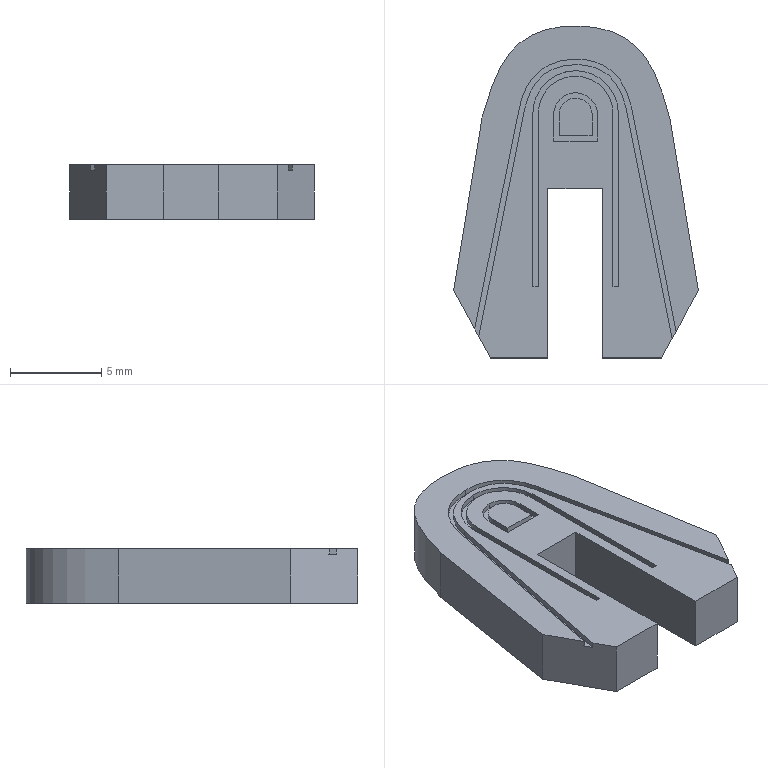Part | SolidWorks | features BaseBody 1 | 1 solid | 46 faces | box 13.412 x 18.194 x 3 mm | volume 493.747 mm3 | plane 29 | spline 17